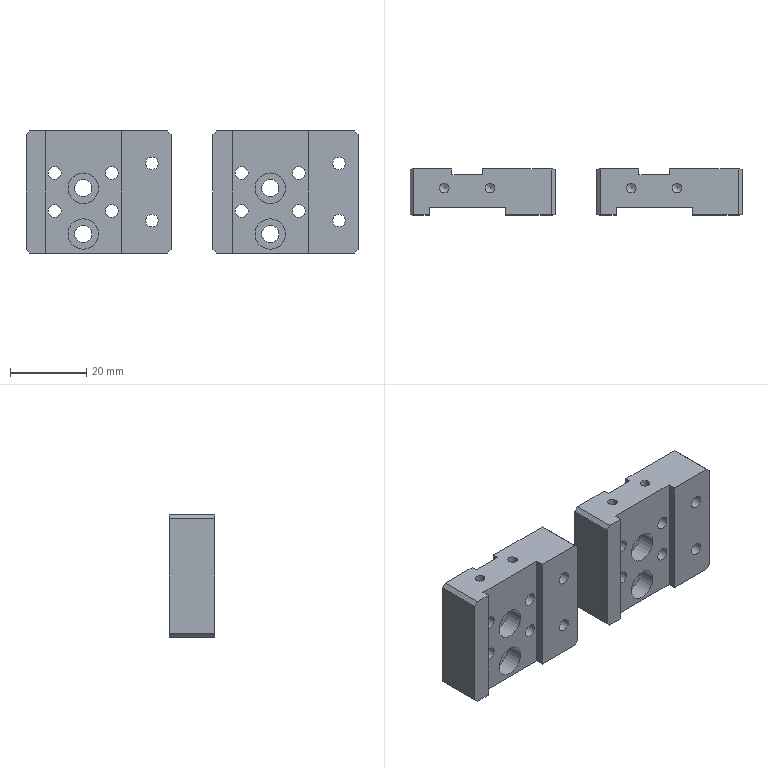CAM job | NX | 3+2 milling, drilling | part box 87 x 12 x 32 mm | stock box 92 x 15 x 37 mm
Tools:
number,name,description,diameter,corner_radius,flute_length,length,flutes
4,D4,平底铣刀-粗,4.0,0.0,25.0,75.0,2
6,D6,平底铣刀-粗,6.0,0.0,25.0,75.0,2
9,D10,平底铣刀-粗,10.0,0.0,35.0,75.0,2
11,D4-J,平底铣刀-精,4.0,0.0,50.0,75.0,2
7,D6-J,平底铣刀-精,6.0,0.0,25.0,75.0,2
10,D10-J,平底铣刀-精,10.0,0.0,35.0,75.0,2
1,D80R0.8飞刀,圆鼻刀-粗,80.0,0.8,50.0,75.0,2
1,D80R0.8飞刀-J,圆鼻刀-精,80.0,0.8,50.0,75.0,2
2,D6倒角刀,倒角刀,6.0,0.0,3.0,25.0,2
21,M4X0.7,丝锥,3.3,0.0,35.0,50.0,2
13,ZT3.4,钻头,3.4,0.0,35.0,50.0,2
11,ZT4.5,钻头,4.5,0.0,35.0,50.0,2
13,钻头3.3,Twist Drill 3.3 mm,3.3,0.0,35.0,35.008,2
Operations:
program,operation,operation_type,tool,method,geometry_group,spindle_rpm,surface_speed,feed_per_tooth,feed_cut,feed_plunge,cut_length_mm,path_length_mm,cut_time_min,machine_time_min
B,底壁铣飞面一刀开粗_COPY,VolumeBased25DMillingOperation,D80R0.8飞刀,分层开粗-切深K-步距G,W-B,2800.0,703.696,0.5357,3000.0,100.0,1171.164,2230.186,0.3904,0.4963
B,底壁铣飞面一刀精光_COPY,VolumeBased25DMillingOperation,D80R0.8飞刀-J,侧刃精光-切深K-步距G,W-B,4000.0,1005.28,0.125,1000.0,100.0,194.998,230.998,0.195,0.1986
B,底壁铣分层开粗-中_COPY,VolumeBased25DMillingOperation,D10,分层开粗-切深K-步距G,W-B,8000.0,251.32,0.25,4000.0,100.0,1511.605,1613.758,0.3779,0.3881
B,COUNTERBORE_1,CylinderMilling,D4,METHOD,W-B,8000.0,100.531,0.1125,1800.0,100.0,752.129,1018.329,0.4178,0.4445
B,BORE_1,CylinderMilling,D4-J,METHOD,W-B,8000.0,100.531,0.0375,600.0,100.0,70.071,355.871,0.1168,0.1454
B,底壁铣精光底面-中_COPY,VolumeBased25DMillingOperation,D10-J,精光步距切深关,W-B,8000.0,251.32,0.0625,1000.0,100.0,206.733,282.335,0.2067,0.2143
B,钻倒角_2,Operation,D6倒角刀,METHOD,W-B,8000.0,150.796,0.0625,1000.0,0.0,20.8,170.286,0.0208,0.0357
B,平面去毛刺6X45L_COPY,SurfaceContour,D6倒角刀,爬面_倒角-切深0-步距G,W-B,6500.0,122.519,0.1154,1500.0,100.0,554.948,1256.434,0.37,0.4401
B,底壁铣精光侧面-中-选底面_COPY,VolumeBased25DMillingOperation,D10-J,侧刃精光-切深K-步距G,W-B,8000.0,251.32,0.0625,1000.0,100.0,208.67,286.914,0.2087,0.2165
A,顶面开粗,FaceMilling,D80R0.8飞刀,分层开粗-切深K-步距G,W-A,4000.0,1005.31,0.375,3000.0,100.0,181.0,216.8,0.0603,0.0639
A,顶面,FaceMilling,D80R0.8飞刀,侧刃精光-切深K-步距G,W-A,4000.0,1005.31,0.125,1000.0,100.0,181.0,217.0,0.181,0.1846
A,外形粗_2,VolumeBased25DMillingOperation,D10,METHOD,W-A,8000.0,251.327,0.3125,5000.0,80.0,9166.896,9316.796,1.833,1.848
A,台阶粗_2,CavityMilling,D6,METHOD,W-A,6000.0,188.0,0.25,3500.0,100.0,2518.767,2877.981,0.7196,0.7556
A,底壁粗_1,VolumeBased25DMillingOperation,D6,METHOD,W-A,6000.0,113.0,0.2083,3500.0,100.0,616.0,864.741,0.176,0.2009
A,打点-深0.8,Operation,D6倒角刀,NONE,W-A,8000.0,150.796,0.0312,500.0,90.0,28.8,295.158,0.0576,0.0842
A,通孔-M4螺纹底孔,Operation,钻头3.3,NONE,W-A,3000.0,31.102,0.05,300.0,90.0,49.966,235.008,0.1666,0.1851
A,沉头孔-钻孔0段,Operation,ZT3.4,NONE,W-A,2800.0,29.908,0.0179,100.0,90.0,112.172,375.624,1.122,1.148
A,通孔-5-6,Operation,ZT4.5,NONE,W-A,3000.0,42.411,0.025,150.0,90.0,52.0,223.093,0.3467,0.3638
A,铣孔开粗D4_1,CylinderMilling,D4,NONE,W-A,8000.0,100.531,0.075,1200.0,100.0,1147.385,1607.385,0.9562,1.002
A,铣孔精光D4_1,CylinderMilling,D4-J,精光步距切深关,W-A,8000.0,100.531,0.0312,500.0,100.0,175.484,635.484,0.351,0.397
A,清角D4,ZLevelMilling,D4-J,METHOD,W-A,6000.0,75.0,0.25,2500.0,80.0,1230.859,1425.766,0.4928,0.5123
A,底精_2,VolumeBased25DMillingOperation,D4-J,METHOD,W-A,6000.0,113.0,0.2083,1200.0,100.0,221.926,374.928,0.1849,0.2002
A,仅选体,SurfaceContour,D6倒角刀,METHOD,W-A,8000.0,150.796,0.1875,3000.0,100.0,616.544,1184.693,0.2055,0.2623
A,钻倒角_1,Operation,D6倒角刀,METHOD,W-A,8000.0,150.796,0.0312,500.0,0.0,20.8,183.286,0.0416,0.0578
A,铣倒角_1,PlanarMilling,D6倒角刀,METHOD,W-A,8000.0,150.796,0.0312,500.0,100.0,69.412,317.413,0.1388,0.1636
A,铣倒角_2,PlanarMilling,D6倒角刀,NONE,W-A,8000.0,150.796,0.0312,500.0,100.0,234.043,625.058,0.4681,0.5072
A,通孔-攻牙M4,Operation,M4X0.7,METHOD,W-A,600.0,6.22,0.0006,0.7,90.0,38.0,211.077,54.286,54.303
A,底侧精_3,VolumeBased25DMillingOperation,D6-J,METHOD,W-A,6000.0,113.0,0.2083,1200.0,100.0,165.226,298.096,0.1377,0.151
A,底侧精_4,VolumeBased25DMillingOperation,D4-J,METHOD,W-A,6000.0,113.0,0.2083,1200.0,100.0,101.561,258.049,0.0846,0.1003
A,外形半精_2,VolumeBased25DMillingOperation,D10-J,METHOD,W-A,8000.0,251.327,0.0625,1000.0,100.0,357.346,420.746,0.3573,0.3637